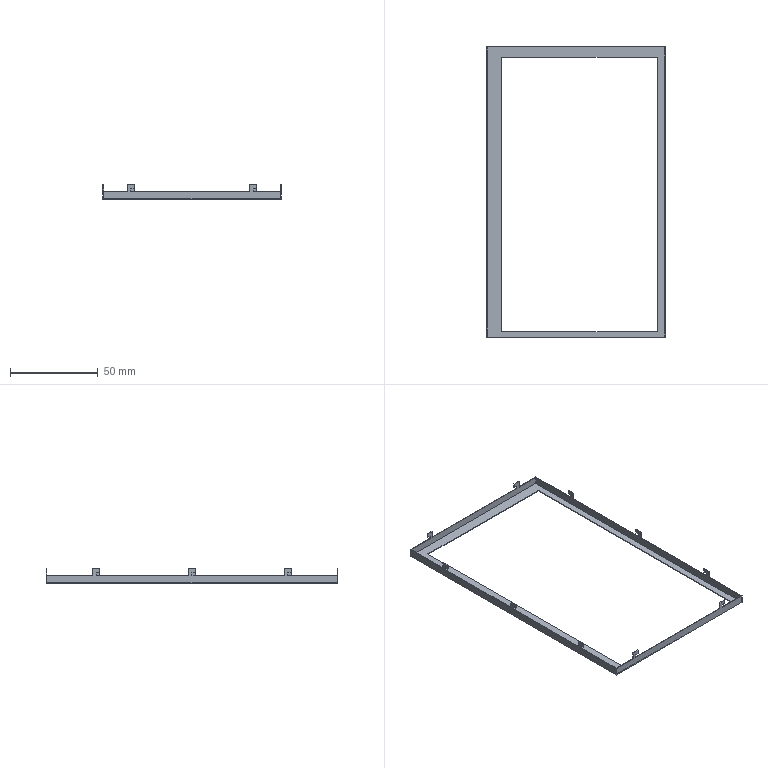Part | STEP file | DMG10600T070_01WTC_X2_8FEA658_4 | 1 solid | 74 faces | box 101.5 x 166.2 x 8.5 mm | volume 2112 mm3 | plane 74